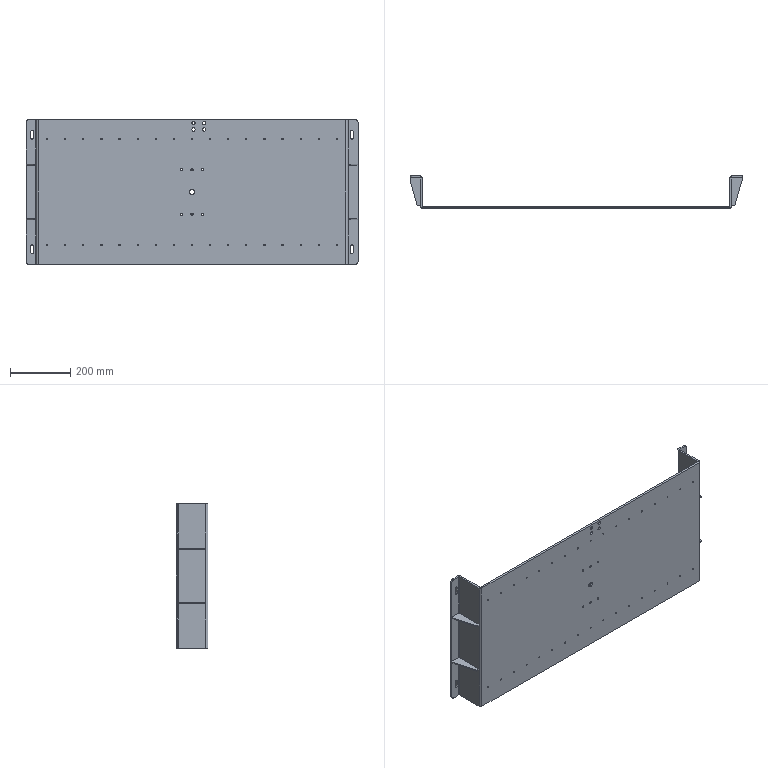Part | SolidWorks | features BaseBody 1 | 1 solid | 244 faces | box 1100 x 106 x 480 mm | volume 3744615 mm3 | cylinder 114 | cone 68 | plane 62 | commonest cylinder face diameters 4.2 x68 7 x12 2 x8 9 x8 11 x8 14 x4